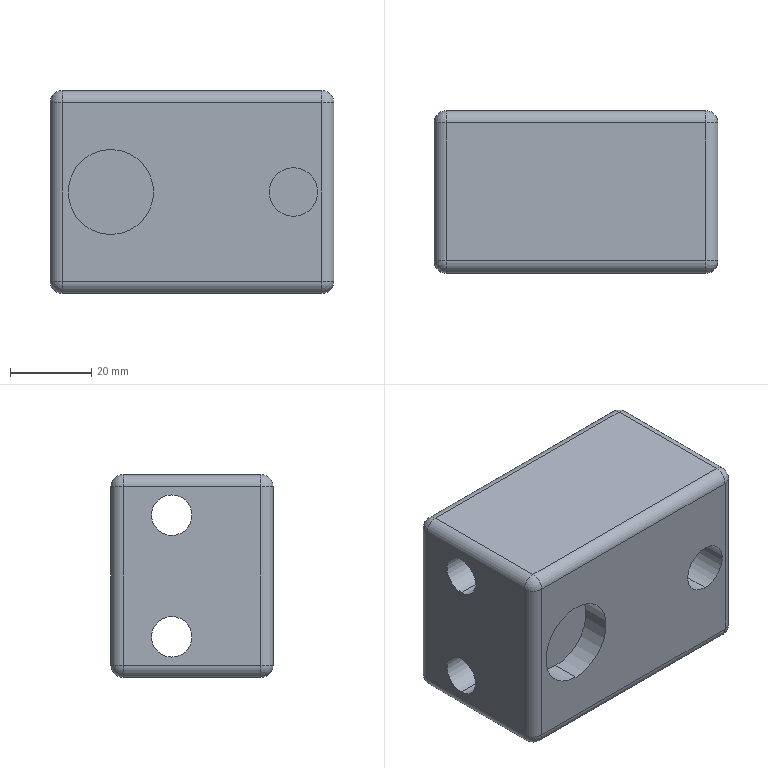Part | SolidWorks | features ICE 3, Extrusion 1, Fillet 1 | 1 solid | 36 faces | box 70 x 40 x 50 mm | volume 121422 mm3 | cylinder 20 | plane 8 | sphere 8 | commonest cylinder face diameters 6 x12 10 x4 12 x2 21 x2
STEP:
#1=CARTESIAN_POINT('',(15.,7.,-14.5));
#2=VERTEX_POINT('',#1);
#3=CARTESIAN_POINT('',(15.,7.,-35.5));
#4=VERTEX_POINT('',#3);
#5=CARTESIAN_POINT('',(15.,7.,-25.));
#6=DIRECTION('',(0.,-1.,0.));
#7=DIRECTION('',(0.,0.,-1.));
#8=AXIS2_PLACEMENT_3D('',#5,#6,#7);
#9=CIRCLE('',#8,10.5);
#10=EDGE_CURVE('',#2,#4,#9,.T.);
#11=ORIENTED_EDGE('',*,*,#10,.F.);
#12=CARTESIAN_POINT('',(15.,0.,-14.5));
#13=VERTEX_POINT('',#12);
#14=CARTESIAN_POINT('',(15.,7.,-14.5));
#15=DIRECTION('',(0.,-1.,0.));
#16=VECTOR('',#15,1000.);
#17=LINE('',#14,#16);
#18=EDGE_CURVE('',#2,#13,#17,.T.);
#19=ORIENTED_EDGE('',*,*,#18,.T.);
#20=CARTESIAN_POINT('',(15.,0.,-35.5));
#21=VERTEX_POINT('',#20);
#22=CARTESIAN_POINT('',(15.,0.,-25.));
#23=DIRECTION('',(0.,-1.,0.));
#24=DIRECTION('',(0.,0.,-1.));
#25=AXIS2_PLACEMENT_3D('',#22,#23,#24);
#26=CIRCLE('',#25,10.5);
#27=EDGE_CURVE('',#13,#21,#26,.T.);
#28=ORIENTED_EDGE('',*,*,#27,.T.);
#29=CARTESIAN_POINT('',(15.,7.,-35.5));
#30=DIRECTION('',(0.,-1.,0.));
#31=VECTOR('',#30,1000.);
#32=LINE('',#29,#31);
#33=EDGE_CURVE('',#4,#21,#32,.T.);
#34=ORIENTED_EDGE('',*,*,#33,.F.);
#35=EDGE_LOOP('',(#11,#19,#28,#34));
#36=FACE_OUTER_BOUND('',#35,.T.);
#37=CARTESIAN_POINT('',(15.,7.,-25.));
#38=DIRECTION('',(0.,-1.,0.));
#39=DIRECTION('',(0.,0.,-1.));
#40=AXIS2_PLACEMENT_3D('',#37,#38,#39);
#41=CYLINDRICAL_SURFACE('',#40,10.5);
#42=ADVANCED_FACE('',(#36),#41,.F.);
#43=CARTESIAN_POINT('',(60.,35.,-19.));
#44=VERTEX_POINT('',#43);
#45=CARTESIAN_POINT('',(60.,35.,-31.));
#46=VERTEX_POINT('',#45);
#47=CARTESIAN_POINT('',(60.,35.,-25.));
#48=DIRECTION('',(0.,-1.,0.));
#49=DIRECTION('',(0.,0.,-1.));
#50=AXIS2_PLACEMENT_3D('',#47,#48,#49);
#51=CIRCLE('',#50,6.);
#52=EDGE_CURVE('',#44,#46,#51,.T.);
#53=ORIENTED_EDGE('',*,*,#52,.F.);
#54=CARTESIAN_POINT('',(60.,0.,-19.));
#55=VERTEX_POINT('',#54);
#56=CARTESIAN_POINT('',(60.,35.,-19.));
#57=DIRECTION('',(0.,-1.,0.));
#58=VECTOR('',#57,1000.);
#59=LINE('',#56,#58);
#60=EDGE_CURVE('',#44,#55,#59,.T.);
#61=ORIENTED_EDGE('',*,*,#60,.T.);
#62=CARTESIAN_POINT('',(60.,0.,-31.));
#63=VERTEX_POINT('',#62);
#64=CARTESIAN_POINT('',(60.,0.,-25.));
#65=DIRECTION('',(0.,-1.,0.));
#66=DIRECTION('',(0.,0.,-1.));
#67=AXIS2_PLACEMENT_3D('',#64,#65,#66);
#68=CIRCLE('',#67,6.);
#69=EDGE_CURVE('',#55,#63,#68,.T.);
#70=ORIENTED_EDGE('',*,*,#69,.T.);
#71=CARTESIAN_POINT('',(60.,35.,-31.));
#72=DIRECTION('',(0.,-1.,0.));
#73=VECTOR('',#72,1000.);
#74=LINE('',#71,#73);
#75=EDGE_CURVE('',#46,#63,#74,.T.);
#76=ORIENTED_EDGE('',*,*,#75,.F.);
#77=EDGE_LOOP('',(#53,#61,#70,#76));
#78=FACE_OUTER_BOUND('',#77,.T.);
#79=CARTESIAN_POINT('',(60.,35.,-25.));
#80=DIRECTION('',(0.,-1.,0.));
#81=DIRECTION('',(0.,0.,-1.));
#82=AXIS2_PLACEMENT_3D('',#79,#80,#81);
#83=CYLINDRICAL_SURFACE('',#82,6.);
#84=ADVANCED_FACE('',(#78),#83,.F.);
#85=CARTESIAN_POINT('',(0.,25.,-5.));
#86=VERTEX_POINT('',#85);
#87=CARTESIAN_POINT('',(0.,25.,-15.));
#88=VERTEX_POINT('',#87);
#89=CARTESIAN_POINT('',(0.,25.,-10.));
#90=DIRECTION('',(1.,0.,0.));
#91=DIRECTION('',(0.,0.,-1.));
#92=AXIS2_PLACEMENT_3D('',#89,#90,#91);
#93=CIRCLE('',#92,5.);
#94=EDGE_CURVE('',#86,#88,#93,.T.);
#95=ORIENTED_EDGE('',*,*,#94,.F.);
#96=CARTESIAN_POINT('',(70.,25.,-5.));
#97=VERTEX_POINT('',#96);
#98=CARTESIAN_POINT('',(0.,25.,-5.));
#99=DIRECTION('',(1.,0.,0.));
#100=VECTOR('',#99,1000.);
#101=LINE('',#98,#100);
#102=EDGE_CURVE('',#86,#97,#101,.T.);
#103=ORIENTED_EDGE('',*,*,#102,.T.);
#104=CARTESIAN_POINT('',(70.,25.,-15.));
#105=VERTEX_POINT('',#104);
#106=CARTESIAN_POINT('',(70.,25.,-10.));
#107=DIRECTION('',(1.,0.,0.));
#108=DIRECTION('',(0.,0.,-1.));
#109=AXIS2_PLACEMENT_3D('',#106,#107,#108);
#110=CIRCLE('',#109,5.);
#111=EDGE_CURVE('',#97,#105,#110,.T.);
#112=ORIENTED_EDGE('',*,*,#111,.T.);
#113=CARTESIAN_POINT('',(0.,25.,-15.));
#114=DIRECTION('',(1.,0.,0.));
#115=VECTOR('',#114,1000.);
#116=LINE('',#113,#115);
#117=EDGE_CURVE('',#88,#105,#116,.T.);
#118=ORIENTED_EDGE('',*,*,#117,.F.);
#119=EDGE_LOOP('',(#95,#103,#112,#118));
#120=FACE_OUTER_BOUND('',#119,.T.);
#121=CARTESIAN_POINT('',(0.,25.,-10.));
#122=DIRECTION('',(1.,0.,0.));
#123=DIRECTION('',(0.,0.,-1.));
#124=AXIS2_PLACEMENT_3D('',#121,#122,#123);
#125=CYLINDRICAL_SURFACE('',#124,5.);
#126=ADVANCED_FACE('',(#120),#125,.F.);
#127=CARTESIAN_POINT('',(0.,25.,-35.));
#128=VERTEX_POINT('',#127);
#129=CARTESIAN_POINT('',(0.,25.,-45.));
#130=VERTEX_POINT('',#129);
#131=CARTESIAN_POINT('',(0.,25.,-40.));
#132=DIRECTION('',(1.,0.,0.));
#133=DIRECTION('',(0.,0.,-1.));
#134=AXIS2_PLACEMENT_3D('',#131,#132,#133);
#135=CIRCLE('',#134,5.);
#136=EDGE_CURVE('',#128,#130,#135,.T.);
#137=ORIENTED_EDGE('',*,*,#136,.F.);
#138=CARTESIAN_POINT('',(70.,25.,-35.));
#139=VERTEX_POINT('',#138);
#140=CARTESIAN_POINT('',(0.,25.,-35.));
#141=DIRECTION('',(1.,0.,0.));
#142=VECTOR('',#141,1000.);
#143=LINE('',#140,#142);
#144=EDGE_CURVE('',#128,#139,#143,.T.);
#145=ORIENTED_EDGE('',*,*,#144,.T.);
#146=CARTESIAN_POINT('',(70.,25.,-45.));
#147=VERTEX_POINT('',#146);
#148=CARTESIAN_POINT('',(70.,25.,-40.));
#149=DIRECTION('',(1.,0.,0.));
#150=DIRECTION('',(0.,0.,-1.));
#151=AXIS2_PLACEMENT_3D('',#148,#149,#150);
#152=CIRCLE('',#151,5.);
#153=EDGE_CURVE('',#139,#147,#152,.T.);
#154=ORIENTED_EDGE('',*,*,#153,.T.);
#155=CARTESIAN_POINT('',(0.,25.,-45.));
#156=DIRECTION('',(1.,0.,0.));
#157=VECTOR('',#156,1000.);
#158=LINE('',#155,#157);
#159=EDGE_CURVE('',#130,#147,#158,.T.);
#160=ORIENTED_EDGE('',*,*,#159,.F.);
#161=EDGE_LOOP('',(#137,#145,#154,#160));
#162=FACE_OUTER_BOUND('',#161,.T.);
#163=CARTESIAN_POINT('',(0.,25.,-40.));
#164=DIRECTION('',(1.,0.,0.));
#165=DIRECTION('',(0.,0.,-1.));
#166=AXIS2_PLACEMENT_3D('',#163,#164,#165);
#167=CYLINDRICAL_SURFACE('',#166,5.);
#168=ADVANCED_FACE('',(#162),#167,.F.);
#169=CARTESIAN_POINT('',(0.,3.,-3.));
#170=VERTEX_POINT('',#169);
#171=CARTESIAN_POINT('',(0.,37.,-3.));
#172=VERTEX_POINT('',#171);
#173=CARTESIAN_POINT('',(0.,40.,-3.));
#174=DIRECTION('',(0.,1.,0.));
#175=VECTOR('',#174,1000.);
#176=LINE('',#173,#175);
#177=EDGE_CURVE('',#170,#172,#176,.T.);
#178=ORIENTED_EDGE('',*,*,#177,.T.);
#179=CARTESIAN_POINT('',(0.,37.,-47.));
#180=VERTEX_POINT('',#179);
#181=CARTESIAN_POINT('',(0.,37.,0.));
#182=DIRECTION('',(0.,0.,-1.));
#183=VECTOR('',#182,1000.);
#184=LINE('',#181,#183);
#185=EDGE_CURVE('',#172,#180,#184,.T.);
#186=ORIENTED_EDGE('',*,*,#185,.T.);
#187=CARTESIAN_POINT('',(0.,3.,-47.));
#188=VERTEX_POINT('',#187);
#189=CARTESIAN_POINT('',(0.,40.,-47.));
#190=DIRECTION('',(0.,-1.,0.));
#191=VECTOR('',#190,1000.);
#192=LINE('',#189,#191);
#193=EDGE_CURVE('',#180,#188,#192,.T.);
#194=ORIENTED_EDGE('',*,*,#193,.T.);
#195=CARTESIAN_POINT('',(0.,3.,0.));
#196=DIRECTION('',(0.,0.,1.));
#197=VECTOR('',#196,1000.);
#198=LINE('',#195,#197);
#199=EDGE_CURVE('',#188,#170,#198,.T.);
#200=ORIENTED_EDGE('',*,*,#199,.T.);
#201=EDGE_LOOP('',(#178,#186,#194,#200));
#202=FACE_OUTER_BOUND('',#201,.T.);
#203=CARTESIAN_POINT('',(0.,25.,-10.));
#204=DIRECTION('',(1.,0.,0.));
#205=DIRECTION('',(0.,0.,-1.));
#206=AXIS2_PLACEMENT_3D('',#203,#204,#205);
#207=CIRCLE('',#206,5.);
#208=EDGE_CURVE('',#88,#86,#207,.T.);
#209=ORIENTED_EDGE('',*,*,#208,.T.);
#210=ORIENTED_EDGE('',*,*,#94,.T.);
#211=EDGE_LOOP('',(#209,#210));
#212=FACE_BOUND('',#211,.T.);
#213=CARTESIAN_POINT('',(0.,25.,-40.));
#214=DIRECTION('',(1.,0.,0.));
#215=DIRECTION('',(0.,0.,-1.));
#216=AXIS2_PLACEMENT_3D('',#213,#214,#215);
#217=CIRCLE('',#216,5.);
#218=EDGE_CURVE('',#130,#128,#217,.T.);
#219=ORIENTED_EDGE('',*,*,#218,.T.);
#220=ORIENTED_EDGE('',*,*,#136,.T.);
#221=EDGE_LOOP('',(#219,#220));
#222=FACE_BOUND('',#221,.T.);
#223=CARTESIAN_POINT('',(0.,40.,0.));
#224=DIRECTION('',(1.,0.,0.));
#225=DIRECTION('',(0.,0.,-1.));
#226=AXIS2_PLACEMENT_3D('',#223,#224,#225);
#227=PLANE('',#226);
#228=ADVANCED_FACE('',(#202,#212,#222),#227,.F.);
#229=CARTESIAN_POINT('',(67.,3.,0.));
#230=VERTEX_POINT('',#229);
#231=CARTESIAN_POINT('',(67.,37.,0.));
#232=VERTEX_POINT('',#231);
#233=CARTESIAN_POINT('',(67.,40.,0.));
#234=DIRECTION('',(0.,1.,0.));
#235=VECTOR('',#234,1000.);
#236=LINE('',#233,#235);
#237=EDGE_CURVE('',#230,#232,#236,.T.);
#238=ORIENTED_EDGE('',*,*,#237,.T.);
#239=CARTESIAN_POINT('',(3.,37.,0.));
#240=VERTEX_POINT('',#239);
#241=CARTESIAN_POINT('',(0.,37.,0.));
#242=DIRECTION('',(-1.,0.,0.));
#243=VECTOR('',#242,1000.);
#244=LINE('',#241,#243);
#245=EDGE_CURVE('',#232,#240,#244,.T.);
#246=ORIENTED_EDGE('',*,*,#245,.T.);
#247=CARTESIAN_POINT('',(3.,3.,0.));
#248=VERTEX_POINT('',#247);
#249=CARTESIAN_POINT('',(3.,40.,0.));
#250=DIRECTION('',(0.,-1.,0.));
#251=VECTOR('',#250,1000.);
#252=LINE('',#249,#251);
#253=EDGE_CURVE('',#240,#248,#252,.T.);
#254=ORIENTED_EDGE('',*,*,#253,.T.);
#255=CARTESIAN_POINT('',(70.,3.,0.));
#256=DIRECTION('',(1.,0.,0.));
#257=VECTOR('',#256,1000.);
#258=LINE('',#255,#257);
#259=EDGE_CURVE('',#248,#230,#258,.T.);
#260=ORIENTED_EDGE('',*,*,#259,.T.);
#261=EDGE_LOOP('',(#238,#246,#254,#260));
#262=FACE_OUTER_BOUND('',#261,.T.);
#263=CARTESIAN_POINT('',(0.,40.,0.));
#264=DIRECTION('',(0.,0.,-1.));
#265=DIRECTION('',(-1.,0.,0.));
#266=AXIS2_PLACEMENT_3D('',#263,#264,#265);
#267=PLANE('',#266);
#268=ADVANCED_FACE('',(#262),#267,.F.);
#269=CARTESIAN_POINT('',(70.,3.,-47.));
#270=VERTEX_POINT('',#269);
#271=CARTESIAN_POINT('',(70.,37.,-47.));
#272=VERTEX_POINT('',#271);
#273=CARTESIAN_POINT('',(70.,40.,-47.));
#274=DIRECTION('',(0.,1.,0.));
#275=VECTOR('',#274,1000.);
#276=LINE('',#273,#275);
#277=EDGE_CURVE('',#270,#272,#276,.T.);
#278=ORIENTED_EDGE('',*,*,#277,.T.);
#279=CARTESIAN_POINT('',(70.,37.,-3.));
#280=VERTEX_POINT('',#279);
#281=CARTESIAN_POINT('',(70.,37.,0.));
#282=DIRECTION('',(0.,0.,1.));
#283=VECTOR('',#282,1000.);
#284=LINE('',#281,#283);
#285=EDGE_CURVE('',#272,#280,#284,.T.);
#286=ORIENTED_EDGE('',*,*,#285,.T.);
#287=CARTESIAN_POINT('',(70.,3.,-3.));
#288=VERTEX_POINT('',#287);
#289=CARTESIAN_POINT('',(70.,40.,-3.));
#290=DIRECTION('',(0.,-1.,0.));
#291=VECTOR('',#290,1000.);
#292=LINE('',#289,#291);
#293=EDGE_CURVE('',#280,#288,#292,.T.);
#294=ORIENTED_EDGE('',*,*,#293,.T.);
#295=CARTESIAN_POINT('',(70.,3.,-50.));
#296=DIRECTION('',(0.,0.,-1.));
#297=VECTOR('',#296,1000.);
#298=LINE('',#295,#297);
#299=EDGE_CURVE('',#288,#270,#298,.T.);
#300=ORIENTED_EDGE('',*,*,#299,.T.);
#301=EDGE_LOOP('',(#278,#286,#294,#300));
#302=FACE_OUTER_BOUND('',#301,.T.);
#303=CARTESIAN_POINT('',(70.,25.,-10.));
#304=DIRECTION('',(1.,0.,0.));
#305=DIRECTION('',(0.,0.,-1.));
#306=AXIS2_PLACEMENT_3D('',#303,#304,#305);
#307=CIRCLE('',#306,5.);
#308=EDGE_CURVE('',#105,#97,#307,.T.);
#309=ORIENTED_EDGE('',*,*,#308,.F.);
#310=ORIENTED_EDGE('',*,*,#111,.F.);
#311=EDGE_LOOP('',(#309,#310));
#312=FACE_BOUND('',#311,.T.);
#313=CARTESIAN_POINT('',(70.,25.,-40.));
#314=DIRECTION('',(1.,0.,0.));
#315=DIRECTION('',(0.,0.,-1.));
#316=AXIS2_PLACEMENT_3D('',#313,#314,#315);
#317=CIRCLE('',#316,5.);
#318=EDGE_CURVE('',#147,#139,#317,.T.);
#319=ORIENTED_EDGE('',*,*,#318,.F.);
#320=ORIENTED_EDGE('',*,*,#153,.F.);
#321=EDGE_LOOP('',(#319,#320));
#322=FACE_BOUND('',#321,.T.);
#323=CARTESIAN_POINT('',(70.,40.,0.));
#324=DIRECTION('',(-1.,0.,0.));
#325=DIRECTION('',(0.,0.,1.));
#326=AXIS2_PLACEMENT_3D('',#323,#324,#325);
#327=PLANE('',#326);
#328=ADVANCED_FACE('',(#302,#312,#322),#327,.F.);
#329=CARTESIAN_POINT('',(3.,3.,-50.));
#330=VERTEX_POINT('',#329);
#331=CARTESIAN_POINT('',(3.,37.,-50.));
#332=VERTEX_POINT('',#331);
#333=CARTESIAN_POINT('',(3.,40.,-50.));
#334=DIRECTION('',(0.,1.,0.));
#335=VECTOR('',#334,1000.);
#336=LINE('',#333,#335);
#337=EDGE_CURVE('',#330,#332,#336,.T.);
#338=ORIENTED_EDGE('',*,*,#337,.T.);
#339=CARTESIAN_POINT('',(67.,37.,-50.));
#340=VERTEX_POINT('',#339);
#341=CARTESIAN_POINT('',(0.,37.,-50.));
#342=DIRECTION('',(1.,0.,0.));
#343=VECTOR('',#342,1000.);
#344=LINE('',#341,#343);
#345=EDGE_CURVE('',#332,#340,#344,.T.);
#346=ORIENTED_EDGE('',*,*,#345,.T.);
#347=CARTESIAN_POINT('',(67.,3.,-50.));
#348=VERTEX_POINT('',#347);
#349=CARTESIAN_POINT('',(67.,40.,-50.));
#350=DIRECTION('',(0.,-1.,0.));
#351=VECTOR('',#350,1000.);
#352=LINE('',#349,#351);
#353=EDGE_CURVE('',#340,#348,#352,.T.);
#354=ORIENTED_EDGE('',*,*,#353,.T.);
#355=CARTESIAN_POINT('',(0.,3.,-50.));
#356=DIRECTION('',(-1.,0.,0.));
#357=VECTOR('',#356,1000.);
#358=LINE('',#355,#357);
#359=EDGE_CURVE('',#348,#330,#358,.T.);
#360=ORIENTED_EDGE('',*,*,#359,.T.);
#361=EDGE_LOOP('',(#338,#346,#354,#360));
#362=FACE_OUTER_BOUND('',#361,.T.);
#363=CARTESIAN_POINT('',(0.,40.,-50.));
#364=DIRECTION('',(0.,0.,1.));
#365=DIRECTION('',(1.,0.,0.));
#366=AXIS2_PLACEMENT_3D('',#363,#364,#365);
#367=PLANE('',#366);
#368=ADVANCED_FACE('',(#362),#367,.F.);
#369=CARTESIAN_POINT('',(67.,40.,-3.));
#370=VERTEX_POINT('',#369);
#371=CARTESIAN_POINT('',(67.,40.,-47.));
#372=VERTEX_POINT('',#371);
#373=CARTESIAN_POINT('',(67.,40.,0.));
#374=DIRECTION('',(0.,0.,-1.));
#375=VECTOR('',#374,1000.);
#376=LINE('',#373,#375);
#377=EDGE_CURVE('',#370,#372,#376,.T.);
#378=ORIENTED_EDGE('',*,*,#377,.T.);
#379=CARTESIAN_POINT('',(3.,40.,-47.));
#380=VERTEX_POINT('',#379);
#381=CARTESIAN_POINT('',(0.,40.,-47.));
#382=DIRECTION('',(-1.,0.,0.));
#383=VECTOR('',#382,1000.);
#384=LINE('',#381,#383);
#385=EDGE_CURVE('',#372,#380,#384,.T.);
#386=ORIENTED_EDGE('',*,*,#385,.T.);
#387=CARTESIAN_POINT('',(3.,40.,-3.));
#388=VERTEX_POINT('',#387);
#389=CARTESIAN_POINT('',(3.,40.,0.));
#390=DIRECTION('',(0.,0.,1.));
#391=VECTOR('',#390,1000.);
#392=LINE('',#389,#391);
#393=EDGE_CURVE('',#380,#388,#392,.T.);
#394=ORIENTED_EDGE('',*,*,#393,.T.);
#395=CARTESIAN_POINT('',(0.,40.,-3.));
#396=DIRECTION('',(1.,0.,0.));
#397=VECTOR('',#396,1000.);
#398=LINE('',#395,#397);
#399=EDGE_CURVE('',#388,#370,#398,.T.);
#400=ORIENTED_EDGE('',*,*,#399,.T.);
#401=EDGE_LOOP('',(#378,#386,#394,#400));
#402=FACE_OUTER_BOUND('',#401,.T.);
#403=CARTESIAN_POINT('',(0.,40.,0.));
#404=DIRECTION('',(0.,-1.,0.));
#405=DIRECTION('',(0.,0.,-1.));
#406=AXIS2_PLACEMENT_3D('',#403,#404,#405);
#407=PLANE('',#406);
#408=ADVANCED_FACE('',(#402),#407,.F.);
#409=CARTESIAN_POINT('',(3.,0.,-47.));
#410=VERTEX_POINT('',#409);
#411=CARTESIAN_POINT('',(67.,0.,-47.));
#412=VERTEX_POINT('',#411);
#413=CARTESIAN_POINT('',(70.,0.,-47.));
#414=DIRECTION('',(1.,0.,0.));
#415=VECTOR('',#414,1000.);
#416=LINE('',#413,#415);
#417=EDGE_CURVE('',#410,#412,#416,.T.);
#418=ORIENTED_EDGE('',*,*,#417,.T.);
#419=CARTESIAN_POINT('',(67.,0.,-3.));
#420=VERTEX_POINT('',#419);
#421=CARTESIAN_POINT('',(67.,0.,0.));
#422=DIRECTION('',(0.,0.,1.));
#423=VECTOR('',#422,1000.);
#424=LINE('',#421,#423);
#425=EDGE_CURVE('',#412,#420,#424,.T.);
#426=ORIENTED_EDGE('',*,*,#425,.T.);
#427=CARTESIAN_POINT('',(3.,0.,-3.));
#428=VERTEX_POINT('',#427);
#429=CARTESIAN_POINT('',(0.,0.,-3.));
#430=DIRECTION('',(-1.,0.,0.));
#431=VECTOR('',#430,1000.);
#432=LINE('',#429,#431);
#433=EDGE_CURVE('',#420,#428,#432,.T.);
#434=ORIENTED_EDGE('',*,*,#433,.T.);
#435=CARTESIAN_POINT('',(3.,0.,-50.));
#436=DIRECTION('',(0.,0.,-1.));
#437=VECTOR('',#436,1000.);
#438=LINE('',#435,#437);
#439=EDGE_CURVE('',#428,#410,#438,.T.);
#440=ORIENTED_EDGE('',*,*,#439,.T.);
#441=EDGE_LOOP('',(#418,#426,#434,#440));
#442=FACE_OUTER_BOUND('',#441,.T.);
#443=CARTESIAN_POINT('',(15.,0.,-25.));
#444=DIRECTION('',(0.,-1.,0.));
#445=DIRECTION('',(0.,0.,-1.));
#446=AXIS2_PLACEMENT_3D('',#443,#444,#445);
#447=CIRCLE('',#446,10.5);
#448=EDGE_CURVE('',#21,#13,#447,.T.);
#449=ORIENTED_EDGE('',*,*,#448,.F.);
#450=ORIENTED_EDGE('',*,*,#27,.F.);
#451=EDGE_LOOP('',(#449,#450));
#452=FACE_BOUND('',#451,.T.);
#453=CARTESIAN_POINT('',(60.,0.,-25.));
#454=DIRECTION('',(0.,-1.,0.));
#455=DIRECTION('',(0.,0.,-1.));
#456=AXIS2_PLACEMENT_3D('',#453,#454,#455);
#457=CIRCLE('',#456,6.);
#458=EDGE_CURVE('',#63,#55,#457,.T.);
#459=ORIENTED_EDGE('',*,*,#458,.F.);
#460=ORIENTED_EDGE('',*,*,#69,.F.);
#461=EDGE_LOOP('',(#459,#460));
#462=FACE_BOUND('',#461,.T.);
#463=CARTESIAN_POINT('',(0.,0.,0.));
#464=DIRECTION('',(0.,-1.,0.));
#465=DIRECTION('',(0.,0.,-1.));
#466=AXIS2_PLACEMENT_3D('',#463,#464,#465);
#467=PLANE('',#466);
#468=ADVANCED_FACE('',(#442,#452,#462),#467,.T.);
#469=ORIENTED_EDGE('',*,*,#144,.F.);
#470=ORIENTED_EDGE('',*,*,#218,.F.);
#471=ORIENTED_EDGE('',*,*,#159,.T.);
#472=ORIENTED_EDGE('',*,*,#318,.T.);
#473=EDGE_LOOP('',(#469,#470,#471,#472));
#474=FACE_OUTER_BOUND('',#473,.T.);
#475=CARTESIAN_POINT('',(0.,25.,-40.));
#476=DIRECTION('',(1.,0.,0.));
#477=DIRECTION('',(0.,0.,-1.));
#478=AXIS2_PLACEMENT_3D('',#475,#476,#477);
#479=CYLINDRICAL_SURFACE('',#478,5.);
#480=ADVANCED_FACE('',(#474),#479,.F.);
#481=ORIENTED_EDGE('',*,*,#102,.F.);
#482=ORIENTED_EDGE('',*,*,#208,.F.);
#483=ORIENTED_EDGE('',*,*,#117,.T.);
#484=ORIENTED_EDGE('',*,*,#308,.T.);
#485=EDGE_LOOP('',(#481,#482,#483,#484));
#486=FACE_OUTER_BOUND('',#485,.T.);
#487=CARTESIAN_POINT('',(0.,25.,-10.));
#488=DIRECTION('',(1.,0.,0.));
#489=DIRECTION('',(0.,0.,-1.));
#490=AXIS2_PLACEMENT_3D('',#487,#488,#489);
#491=CYLINDRICAL_SURFACE('',#490,5.);
#492=ADVANCED_FACE('',(#486),#491,.F.);
#493=ORIENTED_EDGE('',*,*,#60,.F.);
#494=CARTESIAN_POINT('',(60.,35.,-25.));
#495=DIRECTION('',(0.,-1.,0.));
#496=DIRECTION('',(0.,0.,-1.));
#497=AXIS2_PLACEMENT_3D('',#494,#495,#496);
#498=CIRCLE('',#497,6.);
#499=EDGE_CURVE('',#46,#44,#498,.T.);
#500=ORIENTED_EDGE('',*,*,#499,.F.);
#501=ORIENTED_EDGE('',*,*,#75,.T.);
#502=ORIENTED_EDGE('',*,*,#458,.T.);
#503=EDGE_LOOP('',(#493,#500,#501,#502));
#504=FACE_OUTER_BOUND('',#503,.T.);
#505=CARTESIAN_POINT('',(60.,35.,-25.));
#506=DIRECTION('',(0.,-1.,0.));
#507=DIRECTION('',(0.,0.,-1.));
#508=AXIS2_PLACEMENT_3D('',#505,#506,#507);
#509=CYLINDRICAL_SURFACE('',#508,6.);
#510=ADVANCED_FACE('',(#504),#509,.F.);
#511=ORIENTED_EDGE('',*,*,#499,.T.);
#512=ORIENTED_EDGE('',*,*,#52,.T.);
#513=EDGE_LOOP('',(#511,#512));
#514=FACE_OUTER_BOUND('',#513,.T.);
#515=CARTESIAN_POINT('',(60.,35.,-25.));
#516=DIRECTION('',(0.,-1.,0.));
#517=DIRECTION('',(0.,0.,-1.));
#518=AXIS2_PLACEMENT_3D('',#515,#516,#517);
#519=PLANE('',#518);
#520=ADVANCED_FACE('',(#514),#519,.T.);
#521=ORIENTED_EDGE('',*,*,#18,.F.);
#522=CARTESIAN_POINT('',(15.,7.,-25.));
#523=DIRECTION('',(0.,-1.,0.));
#524=DIRECTION('',(0.,0.,-1.));
#525=AXIS2_PLACEMENT_3D('',#522,#523,#524);
#526=CIRCLE('',#525,10.5);
#527=EDGE_CURVE('',#4,#2,#526,.T.);
#528=ORIENTED_EDGE('',*,*,#527,.F.);
#529=ORIENTED_EDGE('',*,*,#33,.T.);
#530=ORIENTED_EDGE('',*,*,#448,.T.);
#531=EDGE_LOOP('',(#521,#528,#529,#530));
#532=FACE_OUTER_BOUND('',#531,.T.);
#533=CARTESIAN_POINT('',(15.,7.,-25.));
#534=DIRECTION('',(0.,-1.,0.));
#535=DIRECTION('',(0.,0.,-1.));
#536=AXIS2_PLACEMENT_3D('',#533,#534,#535);
#537=CYLINDRICAL_SURFACE('',#536,10.5);
#538=ADVANCED_FACE('',(#532),#537,.F.);
#539=ORIENTED_EDGE('',*,*,#527,.T.);
#540=ORIENTED_EDGE('',*,*,#10,.T.);
#541=EDGE_LOOP('',(#539,#540));
#542=FACE_OUTER_BOUND('',#541,.T.);
#543=CARTESIAN_POINT('',(15.,7.,-25.));
#544=DIRECTION('',(0.,-1.,0.));
#545=DIRECTION('',(0.,0.,-1.));
#546=AXIS2_PLACEMENT_3D('',#543,#544,#545);
#547=PLANE('',#546);
#548=ADVANCED_FACE('',(#542),#547,.T.);
#549=CARTESIAN_POINT('',(67.,3.,-3.));
#550=DIRECTION('',(1.,0.,0.));
#551=DIRECTION('',(0.,0.,-1.));
#552=AXIS2_PLACEMENT_3D('',#549,#550,#551);
#553=CIRCLE('',#552,3.);
#554=EDGE_CURVE('',#230,#420,#553,.T.);
#555=ORIENTED_EDGE('',*,*,#554,.F.);
#556=ORIENTED_EDGE('',*,*,#259,.F.);
#557=CARTESIAN_POINT('',(3.,3.,-3.));
#558=DIRECTION('',(-1.,0.,0.));
#559=DIRECTION('',(0.,0.,1.));
#560=AXIS2_PLACEMENT_3D('',#557,#558,#559);
#561=CIRCLE('',#560,3.);
#562=EDGE_CURVE('',#428,#248,#561,.T.);
#563=ORIENTED_EDGE('',*,*,#562,.F.);
#564=ORIENTED_EDGE('',*,*,#433,.F.);
#565=EDGE_LOOP('',(#555,#556,#563,#564));
#566=FACE_OUTER_BOUND('',#565,.T.);
#567=CARTESIAN_POINT('',(0.,3.,-3.));
#568=DIRECTION('',(-1.,0.,0.));
#569=DIRECTION('',(0.,0.,1.));
#570=AXIS2_PLACEMENT_3D('',#567,#568,#569);
#571=CYLINDRICAL_SURFACE('',#570,3.);
#572=ADVANCED_FACE('',(#566),#571,.T.);
#573=CARTESIAN_POINT('',(67.,3.,-3.));
#574=DIRECTION('',(0.,1.,0.));
#575=DIRECTION('',(0.,0.,-1.));
#576=AXIS2_PLACEMENT_3D('',#573,#574,#575);
#577=CIRCLE('',#576,3.);
#578=EDGE_CURVE('',#230,#288,#577,.T.);
#579=ORIENTED_EDGE('',*,*,#578,.F.);
#580=ORIENTED_EDGE('',*,*,#554,.T.);
#581=CARTESIAN_POINT('',(67.,3.,-3.));
#582=DIRECTION('',(0.,0.,-1.));
#583=DIRECTION('',(1.,0.,0.));
#584=AXIS2_PLACEMENT_3D('',#581,#582,#583);
#585=CIRCLE('',#584,3.);
#586=EDGE_CURVE('',#288,#420,#585,.T.);
#587=ORIENTED_EDGE('',*,*,#586,.F.);
#588=EDGE_LOOP('',(#579,#580,#587));
#589=FACE_OUTER_BOUND('',#588,.T.);
#590=CARTESIAN_POINT('',(67.,3.,-3.));
#591=DIRECTION('',(0.,1.,0.));
#592=DIRECTION('',(1.,0.,0.));
#593=AXIS2_PLACEMENT_3D('',#590,#591,#592);
#594=SPHERICAL_SURFACE('',#593,3.);
#595=ADVANCED_FACE('',(#589),#594,.T.);
#596=CARTESIAN_POINT('',(3.,3.,-3.));
#597=DIRECTION('',(0.,0.,-1.));
#598=DIRECTION('',(1.,0.,0.));
#599=AXIS2_PLACEMENT_3D('',#596,#597,#598);
#600=CIRCLE('',#599,3.);
#601=EDGE_CURVE('',#428,#170,#600,.T.);
#602=ORIENTED_EDGE('',*,*,#601,.F.);
#603=ORIENTED_EDGE('',*,*,#562,.T.);
#604=CARTESIAN_POINT('',(3.,3.,-3.));
#605=DIRECTION('',(0.,1.,0.));
#606=DIRECTION('',(0.,0.,-1.));
#607=AXIS2_PLACEMENT_3D('',#604,#605,#606);
#608=CIRCLE('',#607,3.);
#609=EDGE_CURVE('',#170,#248,#608,.T.);
#610=ORIENTED_EDGE('',*,*,#609,.F.);
#611=EDGE_LOOP('',(#602,#603,#610));
#612=FACE_OUTER_BOUND('',#611,.T.);
#613=CARTESIAN_POINT('',(3.,3.,-3.));
#614=DIRECTION('',(0.,1.,0.));
#615=DIRECTION('',(1.,0.,0.));
#616=AXIS2_PLACEMENT_3D('',#613,#614,#615);
#617=SPHERICAL_SURFACE('',#616,3.);
#618=ADVANCED_FACE('',(#612),#617,.T.);
#619=ORIENTED_EDGE('',*,*,#586,.T.);
#620=ORIENTED_EDGE('',*,*,#425,.F.);
#621=CARTESIAN_POINT('',(67.,3.,-47.));
#622=DIRECTION('',(0.,0.,-1.));
#623=DIRECTION('',(-1.,0.,0.));
#624=AXIS2_PLACEMENT_3D('',#621,#622,#623);
#625=CIRCLE('',#624,3.);
#626=EDGE_CURVE('',#270,#412,#625,.T.);
#627=ORIENTED_EDGE('',*,*,#626,.F.);
#628=ORIENTED_EDGE('',*,*,#299,.F.);
#629=EDGE_LOOP('',(#619,#620,#627,#628));
#630=FACE_OUTER_BOUND('',#629,.T.);
#631=CARTESIAN_POINT('',(67.,3.,0.));
#632=DIRECTION('',(0.,0.,1.));
#633=DIRECTION('',(1.,0.,0.));
#634=AXIS2_PLACEMENT_3D('',#631,#632,#633);
#635=CYLINDRICAL_SURFACE('',#634,3.);
#636=ADVANCED_FACE('',(#630),#635,.T.);
#637=ORIENTED_EDGE('',*,*,#578,.T.);
#638=ORIENTED_EDGE('',*,*,#293,.F.);
#639=CARTESIAN_POINT('',(67.,37.,-3.));
#640=DIRECTION('',(0.,1.,0.));
#641=DIRECTION('',(0.,0.,1.));
#642=AXIS2_PLACEMENT_3D('',#639,#640,#641);
#643=CIRCLE('',#642,3.);
#644=EDGE_CURVE('',#232,#280,#643,.T.);
#645=ORIENTED_EDGE('',*,*,#644,.F.);
#646=ORIENTED_EDGE('',*,*,#237,.F.);
#647=EDGE_LOOP('',(#637,#638,#645,#646));
#648=FACE_OUTER_BOUND('',#647,.T.);
#649=CARTESIAN_POINT('',(67.,40.,-3.));
#650=DIRECTION('',(0.,-1.,0.));
#651=DIRECTION('',(0.,0.,-1.));
#652=AXIS2_PLACEMENT_3D('',#649,#650,#651);
#653=CYLINDRICAL_SURFACE('',#652,3.);
#654=ADVANCED_FACE('',(#648),#653,.T.);
#655=CARTESIAN_POINT('',(3.,37.,-3.));
#656=DIRECTION('',(-1.,0.,0.));
#657=DIRECTION('',(0.,0.,1.));
#658=AXIS2_PLACEMENT_3D('',#655,#656,#657);
#659=CIRCLE('',#658,3.);
#660=EDGE_CURVE('',#240,#388,#659,.T.);
#661=ORIENTED_EDGE('',*,*,#660,.F.);
#662=ORIENTED_EDGE('',*,*,#245,.F.);
#663=CARTESIAN_POINT('',(67.,37.,-3.));
#664=DIRECTION('',(1.,0.,0.));
#665=DIRECTION('',(0.,0.,-1.));
#666=AXIS2_PLACEMENT_3D('',#663,#664,#665);
#667=CIRCLE('',#666,3.);
#668=EDGE_CURVE('',#370,#232,#667,.T.);
#669=ORIENTED_EDGE('',*,*,#668,.F.);
#670=ORIENTED_EDGE('',*,*,#399,.F.);
#671=EDGE_LOOP('',(#661,#662,#669,#670));
#672=FACE_OUTER_BOUND('',#671,.T.);
#673=CARTESIAN_POINT('',(0.,37.,-3.));
#674=DIRECTION('',(1.,0.,0.));
#675=DIRECTION('',(0.,0.,-1.));
#676=AXIS2_PLACEMENT_3D('',#673,#674,#675);
#677=CYLINDRICAL_SURFACE('',#676,3.);
#678=ADVANCED_FACE('',(#672),#677,.T.);
#679=ORIENTED_EDGE('',*,*,#609,.T.);
#680=ORIENTED_EDGE('',*,*,#253,.F.);
#681=CARTESIAN_POINT('',(3.,37.,-3.));
#682=DIRECTION('',(0.,1.,0.));
#683=DIRECTION('',(0.,0.,1.));
#684=AXIS2_PLACEMENT_3D('',#681,#682,#683);
#685=CIRCLE('',#684,3.);
#686=EDGE_CURVE('',#172,#240,#685,.T.);
#687=ORIENTED_EDGE('',*,*,#686,.F.);
#688=ORIENTED_EDGE('',*,*,#177,.F.);
#689=EDGE_LOOP('',(#679,#680,#687,#688));
#690=FACE_OUTER_BOUND('',#689,.T.);
#691=CARTESIAN_POINT('',(3.,40.,-3.));
#692=DIRECTION('',(0.,-1.,0.));
#693=DIRECTION('',(0.,0.,-1.));
#694=AXIS2_PLACEMENT_3D('',#691,#692,#693);
#695=CYLINDRICAL_SURFACE('',#694,3.);
#696=ADVANCED_FACE('',(#690),#695,.T.);
#697=ORIENTED_EDGE('',*,*,#601,.T.);
#698=ORIENTED_EDGE('',*,*,#199,.F.);
#699=CARTESIAN_POINT('',(3.,3.,-47.));
#700=DIRECTION('',(0.,0.,-1.));
#701=DIRECTION('',(-1.,0.,0.));
#702=AXIS2_PLACEMENT_3D('',#699,#700,#701);
#703=CIRCLE('',#702,3.);
#704=EDGE_CURVE('',#410,#188,#703,.T.);
#705=ORIENTED_EDGE('',*,*,#704,.F.);
#706=ORIENTED_EDGE('',*,*,#439,.F.);
#707=EDGE_LOOP('',(#697,#698,#705,#706));
#708=FACE_OUTER_BOUND('',#707,.T.);
#709=CARTESIAN_POINT('',(3.,3.,0.));
#710=DIRECTION('',(0.,0.,-1.));
#711=DIRECTION('',(-1.,0.,0.));
#712=AXIS2_PLACEMENT_3D('',#709,#710,#711);
#713=CYLINDRICAL_SURFACE('',#712,3.);
#714=ADVANCED_FACE('',(#708),#713,.T.);
#715=CARTESIAN_POINT('',(67.,3.,-47.));
#716=DIRECTION('',(1.,0.,0.));
#717=DIRECTION('',(0.,0.,-1.));
#718=AXIS2_PLACEMENT_3D('',#715,#716,#717);
#719=CIRCLE('',#718,3.);
#720=EDGE_CURVE('',#412,#348,#719,.T.);
#721=ORIENTED_EDGE('',*,*,#720,.F.);
#722=ORIENTED_EDGE('',*,*,#417,.F.);
#723=CARTESIAN_POINT('',(3.,3.,-47.));
#724=DIRECTION('',(-1.,0.,0.));
#725=DIRECTION('',(0.,0.,1.));
#726=AXIS2_PLACEMENT_3D('',#723,#724,#725);
#727=CIRCLE('',#726,3.);
#728=EDGE_CURVE('',#330,#410,#727,.T.);
#729=ORIENTED_EDGE('',*,*,#728,.F.);
#730=ORIENTED_EDGE('',*,*,#359,.F.);
#731=EDGE_LOOP('',(#721,#722,#729,#730));
#732=FACE_OUTER_BOUND('',#731,.T.);
#733=CARTESIAN_POINT('',(0.,3.,-47.));
#734=DIRECTION('',(1.,0.,0.));
#735=DIRECTION('',(0.,0.,-1.));
#736=AXIS2_PLACEMENT_3D('',#733,#734,#735);
#737=CYLINDRICAL_SURFACE('',#736,3.);
#738=ADVANCED_FACE('',(#732),#737,.T.);
#739=ORIENTED_EDGE('',*,*,#626,.T.);
#740=ORIENTED_EDGE('',*,*,#720,.T.);
#741=CARTESIAN_POINT('',(67.,3.,-47.));
#742=DIRECTION('',(0.,1.,0.));
#743=DIRECTION('',(0.,0.,-1.));
#744=AXIS2_PLACEMENT_3D('',#741,#742,#743);
#745=CIRCLE('',#744,3.);
#746=EDGE_CURVE('',#270,#348,#745,.T.);
#747=ORIENTED_EDGE('',*,*,#746,.F.);
#748=EDGE_LOOP('',(#739,#740,#747));
#749=FACE_OUTER_BOUND('',#748,.T.);
#750=CARTESIAN_POINT('',(67.,3.,-47.));
#751=DIRECTION('',(0.,1.,0.));
#752=DIRECTION('',(1.,0.,0.));
#753=AXIS2_PLACEMENT_3D('',#750,#751,#752);
#754=SPHERICAL_SURFACE('',#753,3.);
#755=ADVANCED_FACE('',(#749),#754,.T.);
#756=ORIENTED_EDGE('',*,*,#668,.T.);
#757=ORIENTED_EDGE('',*,*,#644,.T.);
#758=CARTESIAN_POINT('',(67.,37.,-3.));
#759=DIRECTION('',(0.,0.,-1.));
#760=DIRECTION('',(1.,0.,0.));
#761=AXIS2_PLACEMENT_3D('',#758,#759,#760);
#762=CIRCLE('',#761,3.);
#763=EDGE_CURVE('',#370,#280,#762,.T.);
#764=ORIENTED_EDGE('',*,*,#763,.F.);
#765=EDGE_LOOP('',(#756,#757,#764));
#766=FACE_OUTER_BOUND('',#765,.T.);
#767=CARTESIAN_POINT('',(67.,37.,-3.));
#768=DIRECTION('',(0.,1.,0.));
#769=DIRECTION('',(1.,0.,0.));
#770=AXIS2_PLACEMENT_3D('',#767,#768,#769);
#771=SPHERICAL_SURFACE('',#770,3.);
#772=ADVANCED_FACE('',(#766),#771,.T.);
#773=ORIENTED_EDGE('',*,*,#686,.T.);
#774=ORIENTED_EDGE('',*,*,#660,.T.);
#775=CARTESIAN_POINT('',(3.,37.,-3.));
#776=DIRECTION('',(0.,0.,-1.));
#777=DIRECTION('',(1.,0.,0.));
#778=AXIS2_PLACEMENT_3D('',#775,#776,#777);
#779=CIRCLE('',#778,3.);
#780=EDGE_CURVE('',#172,#388,#779,.T.);
#781=ORIENTED_EDGE('',*,*,#780,.F.);
#782=EDGE_LOOP('',(#773,#774,#781));
#783=FACE_OUTER_BOUND('',#782,.T.);
#784=CARTESIAN_POINT('',(3.,37.,-3.));
#785=DIRECTION('',(0.,1.,0.));
#786=DIRECTION('',(1.,0.,0.));
#787=AXIS2_PLACEMENT_3D('',#784,#785,#786);
#788=SPHERICAL_SURFACE('',#787,3.);
#789=ADVANCED_FACE('',(#783),#788,.T.);
#790=ORIENTED_EDGE('',*,*,#728,.T.);
#791=ORIENTED_EDGE('',*,*,#704,.T.);
#792=CARTESIAN_POINT('',(3.,3.,-47.));
#793=DIRECTION('',(0.,1.,0.));
#794=DIRECTION('',(0.,0.,-1.));
#795=AXIS2_PLACEMENT_3D('',#792,#793,#794);
#796=CIRCLE('',#795,3.);
#797=EDGE_CURVE('',#330,#188,#796,.T.);
#798=ORIENTED_EDGE('',*,*,#797,.F.);
#799=EDGE_LOOP('',(#790,#791,#798));
#800=FACE_OUTER_BOUND('',#799,.T.);
#801=CARTESIAN_POINT('',(3.,3.,-47.));
#802=DIRECTION('',(0.,1.,0.));
#803=DIRECTION('',(1.,0.,0.));
#804=AXIS2_PLACEMENT_3D('',#801,#802,#803);
#805=SPHERICAL_SURFACE('',#804,3.);
#806=ADVANCED_FACE('',(#800),#805,.T.);
#807=ORIENTED_EDGE('',*,*,#746,.T.);
#808=ORIENTED_EDGE('',*,*,#353,.F.);
#809=CARTESIAN_POINT('',(67.,37.,-47.));
#810=DIRECTION('',(0.,1.,0.));
#811=DIRECTION('',(0.,0.,1.));
#812=AXIS2_PLACEMENT_3D('',#809,#810,#811);
#813=CIRCLE('',#812,3.);
#814=EDGE_CURVE('',#272,#340,#813,.T.);
#815=ORIENTED_EDGE('',*,*,#814,.F.);
#816=ORIENTED_EDGE('',*,*,#277,.F.);
#817=EDGE_LOOP('',(#807,#808,#815,#816));
#818=FACE_OUTER_BOUND('',#817,.T.);
#819=CARTESIAN_POINT('',(67.,40.,-47.));
#820=DIRECTION('',(0.,-1.,0.));
#821=DIRECTION('',(0.,0.,-1.));
#822=AXIS2_PLACEMENT_3D('',#819,#820,#821);
#823=CYLINDRICAL_SURFACE('',#822,3.);
#824=ADVANCED_FACE('',(#818),#823,.T.);
#825=ORIENTED_EDGE('',*,*,#763,.T.);
#826=ORIENTED_EDGE('',*,*,#285,.F.);
#827=CARTESIAN_POINT('',(67.,37.,-47.));
#828=DIRECTION('',(0.,0.,-1.));
#829=DIRECTION('',(-1.,0.,0.));
#830=AXIS2_PLACEMENT_3D('',#827,#828,#829);
#831=CIRCLE('',#830,3.);
#832=EDGE_CURVE('',#372,#272,#831,.T.);
#833=ORIENTED_EDGE('',*,*,#832,.F.);
#834=ORIENTED_EDGE('',*,*,#377,.F.);
#835=EDGE_LOOP('',(#825,#826,#833,#834));
#836=FACE_OUTER_BOUND('',#835,.T.);
#837=CARTESIAN_POINT('',(67.,37.,0.));
#838=DIRECTION('',(0.,0.,-1.));
#839=DIRECTION('',(-1.,0.,0.));
#840=AXIS2_PLACEMENT_3D('',#837,#838,#839);
#841=CYLINDRICAL_SURFACE('',#840,3.);
#842=ADVANCED_FACE('',(#836),#841,.T.);
#843=ORIENTED_EDGE('',*,*,#780,.T.);
#844=ORIENTED_EDGE('',*,*,#393,.F.);
#845=CARTESIAN_POINT('',(3.,37.,-47.));
#846=DIRECTION('',(0.,0.,-1.));
#847=DIRECTION('',(-1.,0.,0.));
#848=AXIS2_PLACEMENT_3D('',#845,#846,#847);
#849=CIRCLE('',#848,3.);
#850=EDGE_CURVE('',#180,#380,#849,.T.);
#851=ORIENTED_EDGE('',*,*,#850,.F.);
#852=ORIENTED_EDGE('',*,*,#185,.F.);
#853=EDGE_LOOP('',(#843,#844,#851,#852));
#854=FACE_OUTER_BOUND('',#853,.T.);
#855=CARTESIAN_POINT('',(3.,37.,0.));
#856=DIRECTION('',(0.,0.,1.));
#857=DIRECTION('',(1.,0.,0.));
#858=AXIS2_PLACEMENT_3D('',#855,#856,#857);
#859=CYLINDRICAL_SURFACE('',#858,3.);
#860=ADVANCED_FACE('',(#854),#859,.T.);
#861=ORIENTED_EDGE('',*,*,#797,.T.);
#862=ORIENTED_EDGE('',*,*,#193,.F.);
#863=CARTESIAN_POINT('',(3.,37.,-47.));
#864=DIRECTION('',(0.,1.,0.));
#865=DIRECTION('',(0.,0.,1.));
#866=AXIS2_PLACEMENT_3D('',#863,#864,#865);
#867=CIRCLE('',#866,3.);
#868=EDGE_CURVE('',#332,#180,#867,.T.);
#869=ORIENTED_EDGE('',*,*,#868,.F.);
#870=ORIENTED_EDGE('',*,*,#337,.F.);
#871=EDGE_LOOP('',(#861,#862,#869,#870));
#872=FACE_OUTER_BOUND('',#871,.T.);
#873=CARTESIAN_POINT('',(3.,40.,-47.));
#874=DIRECTION('',(0.,-1.,0.));
#875=DIRECTION('',(0.,0.,-1.));
#876=AXIS2_PLACEMENT_3D('',#873,#874,#875);
#877=CYLINDRICAL_SURFACE('',#876,3.);
#878=ADVANCED_FACE('',(#872),#877,.T.);
#879=ORIENTED_EDGE('',*,*,#832,.T.);
#880=ORIENTED_EDGE('',*,*,#814,.T.);
#881=CARTESIAN_POINT('',(67.,37.,-47.));
#882=DIRECTION('',(-1.,0.,0.));
#883=DIRECTION('',(0.,0.,-1.));
#884=AXIS2_PLACEMENT_3D('',#881,#882,#883);
#885=CIRCLE('',#884,3.);
#886=EDGE_CURVE('',#372,#340,#885,.T.);
#887=ORIENTED_EDGE('',*,*,#886,.F.);
#888=EDGE_LOOP('',(#879,#880,#887));
#889=FACE_OUTER_BOUND('',#888,.T.);
#890=CARTESIAN_POINT('',(67.,37.,-47.));
#891=DIRECTION('',(0.,1.,0.));
#892=DIRECTION('',(1.,0.,0.));
#893=AXIS2_PLACEMENT_3D('',#890,#891,#892);
#894=SPHERICAL_SURFACE('',#893,3.);
#895=ADVANCED_FACE('',(#889),#894,.T.);
#896=ORIENTED_EDGE('',*,*,#868,.T.);
#897=ORIENTED_EDGE('',*,*,#850,.T.);
#898=CARTESIAN_POINT('',(3.,37.,-47.));
#899=DIRECTION('',(1.,0.,0.));
#900=DIRECTION('',(0.,0.,1.));
#901=AXIS2_PLACEMENT_3D('',#898,#899,#900);
#902=CIRCLE('',#901,3.);
#903=EDGE_CURVE('',#332,#380,#902,.T.);
#904=ORIENTED_EDGE('',*,*,#903,.F.);
#905=EDGE_LOOP('',(#896,#897,#904));
#906=FACE_OUTER_BOUND('',#905,.T.);
#907=CARTESIAN_POINT('',(3.,37.,-47.));
#908=DIRECTION('',(0.,1.,0.));
#909=DIRECTION('',(1.,0.,0.));
#910=AXIS2_PLACEMENT_3D('',#907,#908,#909);
#911=SPHERICAL_SURFACE('',#910,3.);
#912=ADVANCED_FACE('',(#906),#911,.T.);
#913=ORIENTED_EDGE('',*,*,#886,.T.);
#914=ORIENTED_EDGE('',*,*,#345,.F.);
#915=ORIENTED_EDGE('',*,*,#903,.T.);
#916=ORIENTED_EDGE('',*,*,#385,.F.);
#917=EDGE_LOOP('',(#913,#914,#915,#916));
#918=FACE_OUTER_BOUND('',#917,.T.);
#919=CARTESIAN_POINT('',(0.,37.,-47.));
#920=DIRECTION('',(-1.,0.,0.));
#921=DIRECTION('',(0.,0.,1.));
#922=AXIS2_PLACEMENT_3D('',#919,#920,#921);
#923=CYLINDRICAL_SURFACE('',#922,3.);
#924=ADVANCED_FACE('',(#918),#923,.T.);
#925=CLOSED_SHELL('',(#42,#84,#126,#168,#228,#268,#328,#368,#408,#468,#480,#492,#510,#520,#538,#548,#572,#595,#618,#636,#654,#678,#696,#714,#738,#755,#772,#789,#806,#824,#842,#860,#878,#895,#912,#924));
#926=MANIFOLD_SOLID_BREP('',#925);
#927=CARTESIAN_POINT('',(0.,0.,0.));
#928=DIRECTION('',(0.,0.,1.));
#929=DIRECTION('',(1.,0.,0.));
#930=AXIS2_PLACEMENT_3D('',#927,#928,#929);
#931=(LENGTH_UNIT()NAMED_UNIT(*)SI_UNIT(.MILLI.,.METRE.));
#932=UNCERTAINTY_MEASURE_WITH_UNIT(LENGTH_MEASURE(0.00001),#931,'','');
#933=(NAMED_UNIT(*)PLANE_ANGLE_UNIT()SI_UNIT($,.RADIAN.));
#934=(NAMED_UNIT(*)SI_UNIT($,.STERADIAN.)SOLID_ANGLE_UNIT());
#935=(GEOMETRIC_REPRESENTATION_CONTEXT(3)GLOBAL_UNCERTAINTY_ASSIGNED_CONTEXT((#932))GLOBAL_UNIT_ASSIGNED_CONTEXT((#931,#933,#934))REPRESENTATION_CONTEXT('',''));
#936=ADVANCED_BREP_SHAPE_REPRESENTATION('',(#926,#930),#935);